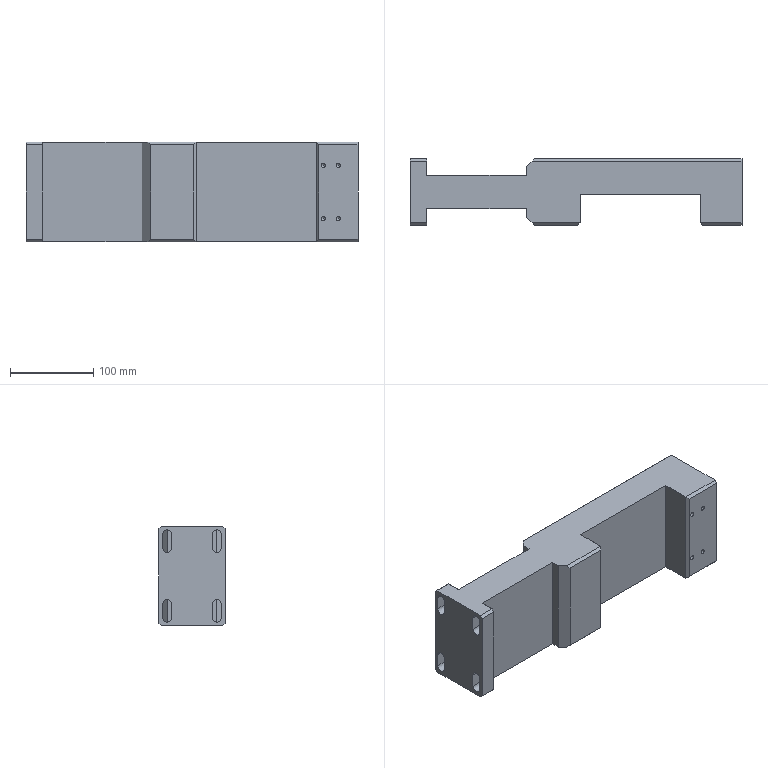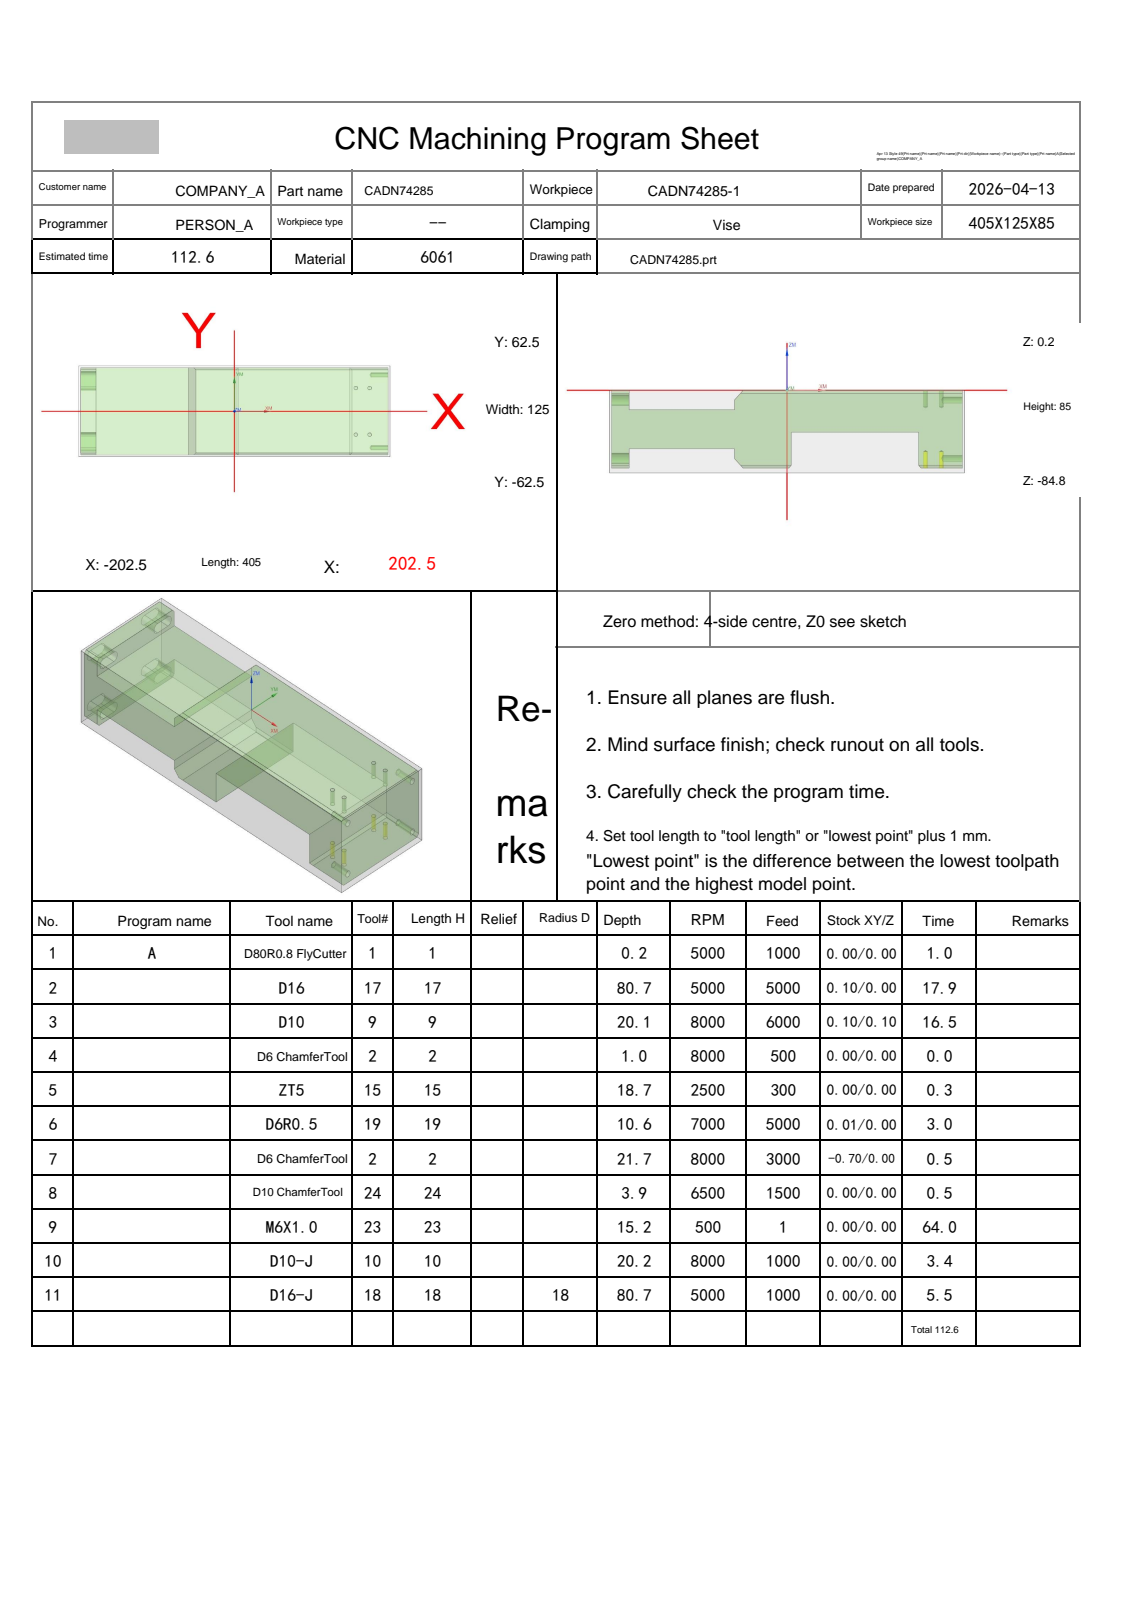NC program | NX | posted by the shop | part box 400 x 80 x 120 mm
Lines 711 to 1887 of 8047:
N3 T09 M06
(D10  D=10. R=0. H=09 ce=0.10 di=0.10)
G00 G90 G54 X-108.23 Y-74.5 M03 S8000
G43 H09 Z10.2
M08
Z.703
G01 Z-.498 F6000.
Y-67.08
G03 X-115.23 Y-60.08 I-7. J0.0
G01 X-174.823
G02 X-175.265 Y-61.98 I-5.294 J.231
X-175.856 Y-63. I-4.852 J2.13
G01 X-176.489
G02 X-180. Y-64.039 I-3.531 J5.482
G01 X-199.92
Y-63.
X-200.
Y-64.039
Y-63.
X-200.08
Y-62.639
X-200.001
X-200. Y-62.64
X-199.999 Y-62.639
X-199.92 Y-62.64
X-198.52 Y-62.639
X-180.
G03 X-174.924 Y-58.018 I-.021 J5.121
G01 X-174.843 Y-57.501
X-174.82 Y-56.969
Y-56.774
X-174.821 Y-56.579
Y-56.188
Y53.513
X-174.82 Y54.405
Y55.297
Y56.188
X-174.822 Y57.085
X-174.844 Y57.509
X-174.924 Y58.018
G03 X-180. Y62.639 I-5.096 J-.499
G01 X-198.52
X-199.92 Y62.64
X-200.08 Y62.639
Y63.
X-199.92
Y64.039
X-179.994
G02 X-176.489 Y63. I-.026 J-6.521
G01 X-175.86
G02 X-174.823 Y60.08 I-4.254 J-3.154
G01 X-174.024
X-65.178
G02 X-64.15 Y63. I5.19 J-.186
G01 X-63.921
X-64.088 Y62.761
X-64.213 Y62.557
X-64.304 Y62.395
X-64.465 Y62.064
X-64.595 Y61.736
X-64.716 Y61.351
X-64.803 Y60.967
X-64.856 Y60.637
X-64.925 Y60.09
X-64.79 Y60.08
X-58.147
G02 X-57.124 Y63. I5.489 J-.285
G01 X-54.085
G02 X-50.568 Y64.039 I3.516 J-5.432
G01 X199.92
Y63.
X200.08
Y62.639
X199.92 Y62.64
X198.52 Y62.639
X-50.568
G03 X-55.639 Y57.568 I0.0 J-5.071
G01 Y-57.568
G03 X-50.568 Y-62.639 I5.071 J0.0
G01 X199.92
X199.921
X200.08
Y-63.
X199.92
Y-64.039
X-50.568
G02 X-54.085 Y-63. I0.0 J6.471
G01 X-57.14
G02 X-57.487 Y-62.469 I4.246 J3.149
G01 X-57.719 Y-62.023
X-57.883 Y-61.559
X-58.102 Y-60.66
X-58.195 Y-60.08
X-64.79
X-64.925 Y-60.09
X-64.856 Y-60.637
X-64.822 Y-60.857
X-64.757 Y-61.187
X-64.668 Y-61.516
X-64.554 Y-61.845
X-64.414 Y-62.175
X-64.244 Y-62.504
X-64.04 Y-62.833
X-63.917 Y-63.
X-64.152
G02 X-65.178 Y-60.08 I4.162 J3.102
G01 X-112.216
G02 X-113.029 Y-59.662 I.001 J1.
G01 X-117.431 Y-53.498
G03 X-118.244 Y-53.08 I-.813 J-.582
G01 X-166.825
G02 X-167.821 Y-52.084 I.004 J1.
G01 Y52.084
G02 X-166.825 Y53.08 I1. J-.004
G01 X-65.055
X-63.635
G02 X-62.639 Y52.084 I-.004 J-1.
G01 Y-52.084
G02 X-63.635 Y-53.08 I-1. J.004
G01 X-65.178
X-112.216
G02 X-113.029 Y-52.662 I.001 J1.
G01 X-117.431 Y-46.498
G03 X-118.244 Y-46.08 I-.813 J-.582
G01 X-159.826
G02 X-160.821 Y-45.085 I.005 J1.
G01 Y45.085
G02 X-159.826 Y46.08 I1. J-.005
G01 X-70.634
G02 X-69.639 Y45.085 I-.005 J-1.
G01 Y-45.085
G02 X-70.634 Y-46.08 I-1. J.005
G01 X-112.216
G02 X-113.029 Y-45.662 I.001 J1.
G01 X-117.431 Y-39.498
G03 X-118.244 Y-39.08 I-.813 J-.582
G01 X-152.826
G02 X-153.821 Y-38.085 I.005 J1.
G01 Y38.085
G02 X-152.826 Y39.08 I1. J-.005
G01 X-77.634
G02 X-76.639 Y38.085 I-.005 J-1.
G01 Y-38.085
G02 X-77.634 Y-39.08 I-1. J.005
G01 X-112.216
G02 X-113.029 Y-38.662 I0.0 J1.
G01 X-117.431 Y-32.498
G03 X-118.244 Y-32.08 I-.813 J-.582
G01 X-145.826
G02 X-146.821 Y-31.085 I.005 J1.
G01 Y31.085
G02 X-145.826 Y32.08 I1. J-.005
G01 X-84.634
G02 X-83.639 Y31.085 I-.005 J-1.
G01 Y-31.085
G02 X-84.634 Y-32.08 I-1. J.005
G01 X-112.216
G02 X-113.029 Y-31.662 I0.0 J1.
G01 X-117.431 Y-25.498
G03 X-118.244 Y-25.08 I-.814 J-.582
G01 X-138.827
G02 X-139.821 Y-24.085 I.005 J1.
G01 Y24.085
G02 X-138.827 Y25.08 I1. J-.005
G01 X-91.634
G02 X-90.639 Y24.085 I-.005 J-1.
G01 Y-24.085
G02 X-91.634 Y-25.08 I-1. J.005
G01 X-112.216
G02 X-113.029 Y-24.662 I0.0 J1.
G01 X-117.431 Y-18.498
G03 X-118.244 Y-18.08 I-.814 J-.582
G01 X-131.827
G02 X-132.821 Y-17.085 I.005 J1.
G01 Y17.085
G02 X-131.827 Y18.08 I1. J-.005
G01 X-98.634
G02 X-97.639 Y17.085 I-.005 J-1.
G01 Y-17.085
G02 X-98.634 Y-18.08 I-1. J.005
G01 X-112.216
G02 X-113.029 Y-17.662 I0.0 J1.
G01 X-117.431 Y-11.499
G03 X-118.244 Y-11.08 I-.814 J-.581
G01 X-124.827
G02 X-125.821 Y-10.085 I.005 J1.
G01 Y10.085
G02 X-124.827 Y11.08 I1. J-.005
G01 X-105.634
G02 X-104.639 Y10.085 I-.005 J-1.
G01 Y-10.085
G02 X-105.634 Y-11.08 I-1. J.005
G01 X-112.216
G02 X-113.029 Y-10.661 I0.0 J1.
G01 X-117.47 Y-4.444
G03 X-118.052 Y-4.053 I-.814 J-.582
G02 X-118.821 Y-3.085 I.231 J.973
G01 Y3.085
G02 X-117.827 Y4.08 I1. J-.005
G01 X-112.634
G02 X-111.639 Y3.085 I-.005 J-1.
G01 Y-3.085
G02 X-112.634 Y-4.08 I-1. J.005
G01 X-115.23
X-115.73
G03 X-122.73 Y-11.08 I0.0 J-7.
G01 Z.703
G00 Z3.
G01 X-108.23 Y-74.5
G00 Z.205
G01 Z-.995
Y-67.08
G03 X-115.23 Y-60.08 I-7. J0.0
G01 X-174.823
G02 X-180.08 Y-65.148 I-5.294 J.231
G01 X-200. Y-65.151
X-200.085 Y-65.156
X-200.08 Y-65.071
Y-63.136
X-199.92
X-180.
G03 X-174.898 Y-58.014 I-.021 J5.122
G01 X-174.9 Y-57.879
X-174.843 Y-57.501
X-174.82 Y-56.969
Y-56.774
X-174.821 Y-56.579
Y-56.188
Y53.513
X-174.82 Y54.405
Y55.297
Y56.188
X-174.822 Y57.085
X-174.844 Y57.509
X-174.9 Y57.879
Y57.995
Y58.016
G03 X-180. Y63.136 I-5.121 J0.0
G01 X-199.92
X-200.
X-200.08
Y65.071
X-200.085 Y65.156
X-200. Y65.151
X-199.742
X-180.08 Y65.142
G02 X-174.823 Y60.08 I-.034 J-5.296
G01 X-65.178
G02 X-63.663 Y63.563 I5.19 J-.186
G01 X-63.563 Y63.663
X-63.503 Y63.727
X-63.447 Y63.66
X-63.385 Y63.615
X-63.438 Y63.56
X-63.529 Y63.429
X-63.71 Y63.267
X-63.836 Y63.113
X-63.964 Y62.943
X-64.088 Y62.761
X-64.213 Y62.557
X-64.304 Y62.395
X-64.465 Y62.064
X-64.595 Y61.736
X-64.716 Y61.351
X-64.803 Y60.967
X-64.856 Y60.637
X-64.925 Y60.09
X-64.79 Y60.08
X-58.147
G02 X-55.897 Y64.236 I5.489 J-.285
X-52.574 Y65.157 I3.324 J-5.531
X-52.279 Y65.151 I0.0 J-6.453
G01 X200.
X200.085 Y65.156
X200.08 Y65.071
Y63.136
X200.
X199.92
X-51.066
G03 X-56.136 Y58.066 I0.0 J-5.071
G01 Y-58.066
G03 X-51.066 Y-63.136 I5.071 J0.0
G01 X199.92
X200.08
Y-64.215
Y-65.071
X200.085 Y-65.156
X200. Y-65.151
X-52.283
X-53.179 Y-65.129
G02 X-57.487 Y-62.469 I.285 J5.279
G01 X-57.719 Y-62.023
X-57.883 Y-61.559
X-58.102 Y-60.66
X-58.195 Y-60.08
X-64.79
X-64.925 Y-60.09
X-64.856 Y-60.637
X-64.822 Y-60.857
X-64.757 Y-61.187
X-64.668 Y-61.516
X-64.554 Y-61.845
X-64.414 Y-62.175
X-64.244 Y-62.504
X-64.04 Y-62.833
X-63.799 Y-63.16
X-63.529 Y-63.428
X-63.512 Y-63.453
X-63.482 Y-63.523
X-63.443 Y-63.597
X-63.521 Y-63.627
X-63.548 Y-63.64
X-63.624 Y-63.68
X-63.655 Y-63.6
X-63.676 Y-63.553
G02 X-65.178 Y-60.08 I3.686 J3.655
G01 X-112.216
G02 X-113.029 Y-59.662 I.001 J1.
G01 X-117.431 Y-53.498
G03 X-118.244 Y-53.08 I-.813 J-.582
G01 X-166.825
G02 X-167.821 Y-52.083 I.003 J1.
G01 Y52.083
G02 X-166.825 Y53.08 I1. J-.003
G01 X-65.055
X-64.133
G02 X-63.136 Y52.083 I-.003 J-1.
G01 Y-52.083
G02 X-64.133 Y-53.08 I-1. J.003
G01 X-65.178
X-112.216
G02 X-113.029 Y-52.662 I.001 J1.
G01 X-117.431 Y-46.498
G03 X-118.244 Y-46.08 I-.813 J-.582
G01 X-159.825
G02 X-160.821 Y-45.084 I.004 J1.
G01 Y45.084
G02 X-159.825 Y46.08 I1. J-.004
G01 X-71.132
G02 X-70.136 Y45.084 I-.004 J-1.
G01 Y-45.084
G02 X-71.132 Y-46.08 I-1. J.004
G01 X-112.216
G02 X-113.029 Y-45.662 I.001 J1.
G01 X-117.431 Y-39.498
G03 X-118.244 Y-39.08 I-.813 J-.582
G01 X-152.826
G02 X-153.821 Y-38.084 I.004 J1.
G01 Y38.084
G02 X-152.826 Y39.08 I1. J-.004
G01 X-78.132
G02 X-77.136 Y38.084 I-.004 J-1.
G01 Y-38.084
G02 X-78.132 Y-39.08 I-1. J.004
G01 X-112.216
G02 X-113.029 Y-38.662 I0.0 J1.
G01 X-117.431 Y-32.498
G03 X-118.244 Y-32.08 I-.813 J-.582
G01 X-145.826
G02 X-146.821 Y-31.085 I.004 J1.
G01 Y31.084
G02 X-145.826 Y32.08 I1. J-.004
G01 X-85.132
G02 X-84.136 Y31.085 I-.004 J-1.
G01 Y-31.084
G02 X-85.132 Y-32.08 I-1. J.004
G01 X-112.216
G02 X-113.029 Y-31.662 I0.0 J1.
G01 X-117.431 Y-25.498
G03 X-118.244 Y-25.08 I-.814 J-.582
G01 X-138.826
G02 X-139.821 Y-24.085 I.005 J1.
G01 Y24.085
G02 X-138.826 Y25.08 I1. J-.005
G01 X-92.132
G02 X-91.136 Y24.085 I-.005 J-1.
G01 Y-24.085
G02 X-92.132 Y-25.08 I-1. J.005
G01 X-112.216
G02 X-113.029 Y-24.662 I0.0 J1.
G01 X-117.431 Y-18.498
G03 X-118.244 Y-18.08 I-.814 J-.582
G01 X-131.826
G02 X-132.821 Y-17.085 I.005 J1.
G01 Y17.085
G02 X-131.826 Y18.08 I1. J-.005
G01 X-99.132
G02 X-98.136 Y17.085 I-.005 J-1.
G01 Y-17.085
G02 X-99.132 Y-18.08 I-1. J.005
G01 X-112.216
G02 X-113.029 Y-17.662 I0.0 J1.
G01 X-117.431 Y-11.498
G03 X-118.244 Y-11.08 I-.814 J-.582
G01 X-124.826
G02 X-125.821 Y-10.085 I.005 J1.
G01 Y10.085
G02 X-124.826 Y11.08 I1. J-.005
G01 X-106.132
G02 X-105.136 Y10.085 I-.005 J-1.
G01 Y-10.085
G02 X-106.132 Y-11.08 I-1. J.005
G01 X-112.216
G02 X-113.029 Y-10.661 I0.0 J1.
G01 X-117.47 Y-4.444
G03 X-118.052 Y-4.053 I-.814 J-.582
G02 X-118.821 Y-3.085 I.231 J.973
G01 Y3.085
G02 X-117.826 Y4.08 I1. J-.005
G01 X-113.131
G02 X-112.136 Y3.085 I-.005 J-1.
G01 Y-3.085
G02 X-113.131 Y-4.08 I-1. J.005
G01 X-115.23
X-115.73
G03 X-122.73 Y-11.08 I0.0 J-7.
G01 Z.205
G00 Z3.
G01 X-108.23 Y-74.5
G00 Z-.293
G01 Z-1.493
Y-67.08
G03 X-115.23 Y-60.08 I-7. J0.0
G01 X-174.823
G02 X-178.055 Y-64.731 I-5.294 J.231
X-180. Y-65.034 I-1.965 J6.218
G01 X-199.92
Y-63.634
X-180.
G03 X-174.9 Y-58.513 I-.021 J5.121
G01 Y-58.492
Y-57.879
X-174.843 Y-57.501
X-174.82 Y-56.969
Y-56.774
X-174.821 Y-56.579
Y-56.188
Y53.513
X-174.82 Y54.405
Y55.297
Y56.188
X-174.822 Y57.085
X-174.844 Y57.509
X-174.9 Y57.879
Y58.492
Y58.513
G03 X-180. Y63.634 I-5.121 J0.0
G01 X-199.92
Y65.034
X-179.994
G02 X-178.105 Y64.746 I-.026 J-6.521
X-174.823 Y60.08 I-2.008 J-4.9
G01 X-65.178
G02 X-64.15 Y63. I5.19 J-.186
G01 X-63.921
X-64.088 Y62.761
X-64.213 Y62.557
X-64.304 Y62.395
X-64.465 Y62.064
X-64.595 Y61.736
X-64.716 Y61.351
X-64.803 Y60.967
X-64.856 Y60.637
X-64.925 Y60.09
X-64.79 Y60.08
X-58.147
G02 X-57.124 Y63. I5.489 J-.285
G01 X-56.273
G02 X-51.563 Y65.034 I4.71 J-4.437
G01 X199.92
Y63.634
X-51.563
G03 X-56.634 Y58.563 I0.0 J-5.071
G01 Y-58.563
G03 X-51.563 Y-63.634 I5.071 J0.0
G01 X199.92
Y-65.034
X-51.563
G02 X-56.273 Y-63. I0.0 J6.471
G01 X-57.14
G02 X-57.487 Y-62.469 I4.246 J3.149
G01 X-57.719 Y-62.023
X-57.883 Y-61.559
X-58.102 Y-60.66
X-58.195 Y-60.08
X-64.79
X-64.925 Y-60.09
X-64.856 Y-60.637
X-64.822 Y-60.857
X-64.757 Y-61.187
X-64.668 Y-61.516
X-64.554 Y-61.845
X-64.414 Y-62.175
X-64.244 Y-62.504
X-64.04 Y-62.833
X-63.917 Y-63.
X-64.152
G02 X-65.178 Y-60.08 I4.162 J3.102
G01 X-112.216
G02 X-113.029 Y-59.662 I.001 J1.
G01 X-117.431 Y-53.499
G03 X-118.244 Y-53.08 I-.813 J-.582
G01 X-166.826
G02 X-167.821 Y-52.085 I.005 J1.
G01 Y52.085
G02 X-166.826 Y53.08 I1. J-.005
G01 X-65.055
X-64.629
G02 X-63.634 Y52.085 I-.005 J-1.
G01 Y-52.085
G02 X-64.629 Y-53.08 I-1. J.005
G01 X-65.068 Y-53.081
X-112.216 Y-53.08
G02 X-113.029 Y-52.662 I.001 J1.
G01 X-117.431 Y-46.499
G03 X-118.244 Y-46.08 I-.813 J-.582
G01 X-159.827
G02 X-160.821 Y-45.085 I.005 J1.
G01 Y45.085
G02 X-159.827 Y46.08 I1. J-.005
G01 X-71.629
G02 X-70.634 Y45.085 I-.005 J-1.
G01 Y-45.086
G02 X-71.629 Y-46.081 I-1. J.005
G01 X-112.216 Y-46.08
G02 X-113.029 Y-45.662 I.001 J1.
G01 X-117.431 Y-39.499
G03 X-118.244 Y-39.08 I-.813 J-.582
G01 X-152.827
G02 X-153.821 Y-38.086 I.006 J1.
G01 Y38.086
G02 X-152.827 Y39.08 I1. J-.006
G01 X-78.628
G02 X-77.634 Y38.086 I-.006 J-1.
G01 Y-38.086
G02 X-78.628 Y-39.081 I-1. J.006
G01 X-112.216 Y-39.08
G02 X-113.029 Y-38.662 I0.0 J1.
G01 X-117.431 Y-32.499
G03 X-118.244 Y-32.08 I-.813 J-.582
G01 X-145.827
G02 X-146.821 Y-31.086 I.006 J1.
G01 Y31.086
G02 X-145.827 Y32.08 I1. J-.006
G01 X-85.628
G02 X-84.634 Y31.086 I-.006 J-1.
G01 Y-31.086
G02 X-85.628 Y-32.081 I-1. J.006
G01 X-112.216 Y-32.08
G02 X-113.029 Y-31.662 I0.0 J1.
G01 X-117.431 Y-25.499
G03 X-118.244 Y-25.08 I-.814 J-.582
G01 X-138.827
G02 X-139.821 Y-24.086 I.006 J1.
G01 Y24.086
G02 X-138.827 Y25.08 I1. J-.006
G01 X-92.628
G02 X-91.634 Y24.086 I-.006 J-1.
G01 Y-24.086
G02 X-92.628 Y-25.081 I-1. J.006
G01 X-112.216 Y-25.08
G02 X-113.029 Y-24.662 I0.0 J1.
G01 X-117.431 Y-18.499
G03 X-118.244 Y-18.08 I-.814 J-.582
G01 X-131.827
G02 X-132.821 Y-17.086 I.006 J1.
G01 Y17.086
G02 X-131.827 Y18.08 I1. J-.006
G01 X-99.628
G02 X-98.634 Y17.086 I-.006 J-1.
G01 Y-17.087
G02 X-99.628 Y-18.081 I-1. J.006
G01 X-112.216 Y-18.08
G02 X-113.029 Y-17.662 I0.0 J1.
G01 X-117.431 Y-11.499
G03 X-118.244 Y-11.08 I-.814 J-.581
G01 X-124.827
G02 X-125.821 Y-10.086 I.006 J1.
G01 Y10.086
G02 X-124.827 Y11.08 I1. J-.006
G01 X-106.628
G02 X-105.634 Y10.086 I-.006 J-1.
G01 Y-10.087
G02 X-106.628 Y-11.081 I-1. J.006
G01 X-112.215 Y-11.08
G02 X-113.029 Y-10.662 I0.0 J1.
G01 X-117.469 Y-4.445
G03 X-118.052 Y-4.054 I-.814 J-.582
G02 X-118.821 Y-3.086 I.23 J.973
G01 Y3.086
G02 X-117.827 Y4.08 I1. J-.006
G01 X-113.628
G02 X-112.634 Y3.086 I-.006 J-1.
G01 Y-3.087
G02 X-113.628 Y-4.08 I-1. J.006
G01 X-115.23
X-115.73
G03 X-122.73 Y-11.08 I0.0 J-7.
G01 Z-.293
G00 Z3.
G01 X-108.23 Y-74.5
G00 Z-.79
G01 Z-1.99
Y-67.08
G03 X-115.23 Y-60.08 I-7. J0.0
G01 X-174.823
G02 X-180.08 Y-65.148 I-5.294 J.231
G01 X-200. Y-65.151
X-200.085 Y-65.156
X-200.08 Y-65.071
Y-64.131
X-199.92
X-180.
G03 X-174.9 Y-58.99 I-.042 J5.142
G01 Y-57.879
X-174.843 Y-57.501
X-174.82 Y-56.969
Y-56.774
X-174.821 Y-56.579
Y-56.188
Y53.513
X-174.82 Y54.405
Y55.297
Y56.188
X-174.822 Y57.085
X-174.844 Y57.509
X-174.9 Y57.879
Y58.99
G03 X-180. Y64.131 I-5.142 J-.001
G01 X-199.92
X-199.997
X-200.
X-200.08
Y65.071
X-200.085 Y65.156
X-200. Y65.151
X-199.742
X-180.08 Y65.142
G02 X-174.823 Y60.08 I-.034 J-5.296
G01 X-65.178
G02 X-63.663 Y63.563 I5.19 J-.186
G01 X-63.563 Y63.663
X-63.503 Y63.727
X-63.447 Y63.66
X-63.385 Y63.615
X-63.438 Y63.56
X-63.529 Y63.429
X-63.71 Y63.267
X-63.836 Y63.113
X-63.964 Y62.943
X-64.088 Y62.761
X-64.213 Y62.557
X-64.304 Y62.395
X-64.465 Y62.064
X-64.595 Y61.736
X-64.716 Y61.351
X-64.803 Y60.967
X-64.856 Y60.637
X-64.925 Y60.09
X-64.79 Y60.08
X-58.147
G02 X-55.897 Y64.236 I5.489 J-.285
X-52.574 Y65.157 I3.324 J-5.531
X-52.279 Y65.151 I0.0 J-6.453
G01 X200.
X200.085 Y65.156
X200.08 Y65.071
Y64.131
X200.
X199.997
X199.92
X-52.061
G03 X-57.131 Y59.061 I0.0 J-5.071
G01 Y-59.061
G03 X-52.061 Y-64.131 I5.071 J0.0
G01 X199.92
X200.08
Y-65.071
X200.085 Y-65.156
X200. Y-65.151
X-52.283
X-53.179 Y-65.129
G02 X-57.487 Y-62.469 I.285 J5.279
G01 X-57.719 Y-62.023
X-57.883 Y-61.559
X-58.102 Y-60.66
X-58.195 Y-60.08
X-64.79
X-64.925 Y-60.09
X-64.856 Y-60.637
X-64.822 Y-60.857
X-64.757 Y-61.187
X-64.668 Y-61.516
X-64.554 Y-61.845
X-64.414 Y-62.175
X-64.244 Y-62.504
X-64.04 Y-62.833
X-63.799 Y-63.16
X-63.529 Y-63.428
X-63.512 Y-63.453
X-63.482 Y-63.523
X-63.443 Y-63.597
X-63.521 Y-63.627
X-63.548 Y-63.64
X-63.624 Y-63.68
X-63.655 Y-63.6
X-63.676 Y-63.553
G02 X-65.178 Y-60.08 I3.686 J3.655
G01 X-112.216
G02 X-113.029 Y-59.662 I.001 J1.
G01 X-117.431 Y-53.498
G03 X-118.244 Y-53.08 I-.813 J-.582
G01 X-166.826
G02 X-167.821 Y-52.084 I.004 J1.
G01 Y52.084
G02 X-166.826 Y53.08 I1. J-.004
G01 X-65.133
X-65.131
G02 X-64.131 Y52.085 I0.0 J-1.
G01 Y-52.085
G02 X-65.132 Y-53.081 I-1.001 J.004
G01 X-65.178 Y-53.08
X-112.216
G02 X-113.029 Y-52.662 I.001 J1.
G01 X-117.431 Y-46.498
G03 X-118.244 Y-46.08 I-.813 J-.582
G01 X-159.826
G02 X-160.821 Y-45.085 I.005 J1.
G01 Y45.085
G02 X-159.826 Y46.08 I1. J-.005
G01 X-72.126
G02 X-71.131 Y45.085 I-.005 J-1.
G01 Y-45.085
G02 X-72.126 Y-46.08 I-1. J.005
G01 X-112.216
G02 X-113.029 Y-45.662 I.001 J1.
G01 X-117.431 Y-39.498
G03 X-118.244 Y-39.08 I-.813 J-.582
G01 X-152.827
G02 X-153.821 Y-38.085 I.005 J1.
G01 Y38.085
G02 X-152.827 Y39.08 I1. J-.005
G01 X-79.126
G02 X-78.131 Y38.085 I-.005 J-1.
G01 Y-38.085
G02 X-79.126 Y-39.08 I-1. J.005
G01 X-112.216
G02 X-113.029 Y-38.662 I0.0 J1.
G01 X-117.431 Y-32.498
G03 X-118.244 Y-32.08 I-.813 J-.582
G01 X-145.827
G02 X-146.821 Y-31.085 I.005 J1.
G01 Y31.085
G02 X-145.827 Y32.08 I1. J-.005
G01 X-86.126
G02 X-85.131 Y31.085 I-.005 J-1.
G01 Y-31.085
G02 X-86.126 Y-32.08 I-1. J.005
G01 X-112.216
G02 X-113.029 Y-31.662 I0.0 J1.
G01 X-117.431 Y-25.498
G03 X-118.244 Y-25.08 I-.814 J-.582
G01 X-138.827
G02 X-139.821 Y-24.085 I.005 J1.
G01 Y24.085
G02 X-138.827 Y25.08 I1. J-.005
G01 X-93.126
G02 X-92.131 Y24.085 I-.005 J-1.
G01 Y-24.085
G02 X-93.126 Y-25.08 I-1. J.005
G01 X-112.216
G02 X-113.029 Y-24.662 I0.0 J1.
G01 X-117.431 Y-18.498
G03 X-118.244 Y-18.08 I-.814 J-.582
G01 X-131.827
G02 X-132.821 Y-17.086 I.006 J1.
G01 Y17.086
G02 X-131.827 Y18.08 I1. J-.006
G01 X-100.126
G02 X-99.131 Y17.086 I-.006 J-1.
G01 Y-17.086
G02 X-100.126 Y-18.08 I-1. J.006
G01 X-112.216
G02 X-113.029 Y-17.662 I0.0 J1.
G01 X-117.431 Y-11.499
G03 X-118.244 Y-11.08 I-.814 J-.581
G01 X-124.827
G02 X-125.821 Y-10.086 I.006 J1.
G01 Y10.086
G02 X-124.827 Y11.08 I1. J-.006
G01 X-107.126
G02 X-106.131 Y10.086 I-.006 J-1.
G01 Y-10.086
G02 X-107.126 Y-11.08 I-1. J.006
G01 X-112.216
G02 X-113.029 Y-10.661 I0.0 J1.
G01 X-117.47 Y-4.444
G03 X-118.052 Y-4.053 I-.814 J-.582
G02 X-118.821 Y-3.086 I.231 J.973
G01 Y3.086
G02 X-117.827 Y4.08 I1. J-.006
G01 X-114.126
G02 X-113.131 Y3.086 I-.006 J-1.
G01 Y-3.086
G02 X-114.126 Y-4.08 I-1. J.006
G01 X-115.23
X-115.73
G03 X-122.73 Y-11.08 I0.0 J-7.
G01 Z-.79
G00 Z3.
G01 X-108.23 Y-74.5
G00 Z-1.288
G01 Z-2.488
Y-67.08
G03 X-115.23 Y-60.08 I-7. J0.0
G01 X-174.823
G02 X-180.08 Y-65.148 I-5.294 J.231
G01 X-200. Y-65.151
X-200.085 Y-65.156
X-200.08 Y-65.071
Y-64.629
X-200.
X-199.991
X-199.92
X-180.
G03 X-174.9 Y-59.487 I-.048 J5.147
G01 Y-57.879
X-174.843 Y-57.501
X-174.82 Y-56.969
Y-56.774
X-174.821 Y-56.579
Y-56.188
Y53.513
X-174.82 Y54.405
Y55.297
Y56.188
X-174.822 Y57.085
X-174.844 Y57.509
X-174.9 Y57.879
Y59.487
G03 X-180. Y64.629 I-5.148 J-.006
G01 X-199.92
X-199.989
X-200.
X-200.08
Y65.071
X-200.085 Y65.156
X-200. Y65.151
X-199.742
X-180.08 Y65.142
G02 X-174.823 Y60.08 I-.034 J-5.296
G01 X-65.178
G02 X-63.663 Y63.563 I5.19 J-.186
G01 X-63.563 Y63.663
X-63.503 Y63.727
X-63.447 Y63.66
X-63.385 Y63.615
X-63.438 Y63.56
X-63.529 Y63.429
X-63.71 Y63.267
X-63.836 Y63.113
X-63.964 Y62.943
X-64.088 Y62.761
X-64.213 Y62.557
X-64.304 Y62.395
X-64.465 Y62.064
X-64.595 Y61.736
X-64.716 Y61.351
X-64.803 Y60.967
X-64.856 Y60.637
X-64.925 Y60.09
X-64.79 Y60.08
X-58.147
G02 X-55.897 Y64.236 I5.489 J-.285
X-52.574 Y65.157 I3.324 J-5.531
X-52.279 Y65.151 I0.0 J-6.453
G01 X200.
X200.085 Y65.156
X200.08 Y65.071
Y64.629
X200.
X199.989
X199.92
X-52.558
G03 X-57.629 Y59.558 I0.0 J-5.071
G01 Y-59.558
G03 X-52.558 Y-64.629 I5.071 J0.0
G01 X199.92
X200.08
Y-65.071
X200.085 Y-65.156
X200. Y-65.151
X-52.283
X-53.179 Y-65.129
G02 X-57.487 Y-62.469 I.285 J5.279
G01 X-57.719 Y-62.023
X-57.883 Y-61.559
X-58.102 Y-60.66
X-58.195 Y-60.08
X-64.79
X-64.925 Y-60.09
X-64.856 Y-60.637
X-64.822 Y-60.857
X-64.757 Y-61.187
X-64.668 Y-61.516
X-64.554 Y-61.845
X-64.414 Y-62.175
X-64.244 Y-62.504
X-64.04 Y-62.833
X-63.799 Y-63.16
X-63.529 Y-63.428
X-63.512 Y-63.453
X-63.482 Y-63.523
X-63.443 Y-63.597
X-63.521 Y-63.627
X-63.548 Y-63.64
X-63.624 Y-63.68
X-63.655 Y-63.6
X-63.676 Y-63.553
G02 X-65.178 Y-60.08 I3.686 J3.655
G01 X-112.216
G02 X-113.029 Y-59.662 I.001 J1.
G01 X-117.431 Y-53.498
G03 X-118.244 Y-53.08 I-.813 J-.582
G01 X-166.826
G02 X-167.821 Y-52.085 I.005 J1.
G01 Y52.085
G02 X-166.826 Y53.08 I1. J-.005
G01 X-65.624
G02 X-64.629 Y52.085 I-.005 J-1.
G01 Y-52.085
G02 X-65.624 Y-53.08 I-1. J.005
G01 X-112.216
G02 X-113.029 Y-52.662 I.001 J1.
G01 X-117.431 Y-46.498
G03 X-118.244 Y-46.08 I-.813 J-.582
G01 X-159.827
G02 X-160.821 Y-45.085 I.005 J1.
G01 Y45.085
G02 X-159.827 Y46.08 I1. J-.005
G01 X-72.624
G02 X-71.629 Y45.085 I-.005 J-1.
G01 Y-45.085
G02 X-72.624 Y-46.08 I-1. J.005
G01 X-112.216
G02 X-113.029 Y-45.662 I.001 J1.
G01 X-117.431 Y-39.498
G03 X-118.244 Y-39.08 I-.813 J-.582
G01 X-152.827
G02 X-153.821 Y-38.085 I.005 J1.
G01 Y38.085
G02 X-152.827 Y39.08 I1. J-.005
G01 X-79.623
G02 X-78.629 Y38.086 I-.005 J-1.
G01 Y-38.086
G02 X-79.623 Y-39.08 I-1. J.005
G01 X-112.216
G02 X-113.029 Y-38.662 I0.0 J1.
G01 X-117.431 Y-32.498
G03 X-118.244 Y-32.08 I-.813 J-.582
G01 X-145.827
G02 X-146.821 Y-31.086 I.006 J1.
G01 Y31.086
G02 X-145.827 Y32.08 I1. J-.006
G01 X-86.623
G02 X-85.629 Y31.086 I-.006 J-1.
G01 Y-31.086
G02 X-86.623 Y-32.08 I-1. J.006
G01 X-112.216
G02 X-113.029 Y-31.662 I0.0 J1.
G01 X-117.431 Y-25.498
G03 X-118.244 Y-25.08 I-.814 J-.582
G01 X-138.827
G02 X-139.821 Y-24.086 I.006 J1.
G01 Y24.086
G02 X-138.827 Y25.08 I1. J-.006
G01 X-93.623
G02 X-92.629 Y24.086 I-.006 J-1.
G01 Y-24.086
G02 X-93.623 Y-25.08 I-1. J.006
G01 X-112.216
G02 X-113.029 Y-24.662 I0.0 J1.
G01 X-117.431 Y-18.498
G03 X-118.244 Y-18.08 I-.814 J-.582
G01 X-131.827
G02 X-132.821 Y-17.086 I.006 J1.
G01 Y17.086
G02 X-131.827 Y18.08 I1. J-.006
G01 X-100.623
G02 X-99.629 Y17.086 I-.006 J-1.
G01 Y-17.086
G02 X-100.623 Y-18.08 I-1. J.006
G01 X-112.216
G02 X-113.029 Y-17.662 I0.0 J1.
G01 X-117.431 Y-11.499
G03 X-118.244 Y-11.08 I-.814 J-.581
G01 X-124.827
G02 X-125.821 Y-10.086 I.006 J1.
G01 Y10.086
G02 X-124.827 Y11.08 I1. J-.006
G01 X-107.623
G02 X-106.629 Y10.086 I-.006 J-1.
G01 Y-10.086
G02 X-107.623 Y-11.08 I-1. J.006
G01 X-112.216
G02 X-113.029 Y-10.661 I0.0 J1.
G01 X-117.47 Y-4.444
G03 X-118.052 Y-4.053 I-.814 J-.582
G02 X-118.821 Y-3.086 I.231 J.973
G01 Y3.086
G02 X-117.827 Y4.08 I1. J-.006
G01 X-114.623
G02 X-113.629 Y3.086 I-.006 J-1.
G01 Y-3.086
G02 X-114.623 Y-4.08 I-1. J.006
G01 X-115.23
X-115.73
G03 X-122.73 Y-11.08 I0.0 J-7.
G01 Z-1.288
G00 Z3.
G01 X-108.23 Y-74.5
G00 Z-1.785
G01 Z-2.985
Y-67.08
G03 X-115.23 Y-60.08 I-7. J0.0
G01 X-174.823
G02 X-175.856 Y-63. I-5.294 J.231
X-176.838 Y-64.012 I-4.26 J3.151
G01 X-176.898 Y-63.939
X-176.479 Y-63.591
X-176.394 Y-63.506
G03 X-174.9 Y-59.9 I-3.606 J3.606
G01 Y-57.879
X-174.843 Y-57.501
X-174.833 Y-57.298
X-174.82 Y-56.969
Y-56.774
X-174.821 Y-56.579
Y-56.188
Y53.513
X-174.82 Y54.405
Y55.297
Y56.188
X-174.822 Y57.085
X-174.832 Y57.293
X-174.844 Y57.509
X-174.9 Y57.879
Y59.9
G03 X-176.394 Y63.506 I-5.1 J0.0
G01 X-176.479 Y63.591
X-176.93 Y63.966
G03 X-177.242 Y64.201 I-3.178 J-3.887
G01 X-177.197 Y64.266
G02 X-175.86 Y63. I-2.917 J-4.42
X-174.823 Y60.08 I-4.254 J-3.154
G01 X-65.178
G02 X-64.15 Y63. I5.19 J-.186
G01 X-63.921
X-64.088 Y62.761
X-64.213 Y62.557
X-64.304 Y62.395
X-64.465 Y62.064
X-64.595 Y61.736
X-64.716 Y61.351
X-64.803 Y60.967
X-64.856 Y60.637
X-64.925 Y60.09
X-64.79 Y60.08
X-58.147
X-58.127 Y59.921
Y59.92
X-58.126 Y-60.037
X-58.195 Y-60.08
X-64.79
X-64.925 Y-60.09
X-64.856 Y-60.637
X-64.822 Y-60.857
X-64.757 Y-61.187
X-64.668 Y-61.516
X-64.554 Y-61.845
X-64.414 Y-62.175
X-64.244 Y-62.504
X-64.04 Y-62.833
X-63.917 Y-63.
X-64.152
G02 X-65.178 Y-60.08 I4.162 J3.102
G01 X-112.216
G02 X-113.029 Y-59.662 I0.0 J1.
G01 X-117.431 Y-53.498
G03 X-118.244 Y-53.08 I-.813 J-.582
G01 X-166.827
G02 X-167.821 Y-52.086 I.006 J1.
G01 Y52.086
G02 X-166.827 Y53.08 I1. J-.006
G01 X-66.121
G02 X-65.126 Y52.086 I-.006 J-1.
G01 Y-52.086
G02 X-66.121 Y-53.08 I-1. J.006
G01 X-112.216
G02 X-113.029 Y-52.662 I.001 J1.
G01 X-117.431 Y-46.498
G03 X-118.244 Y-46.08 I-.813 J-.582
G01 X-159.827
G02 X-160.821 Y-45.086 I.006 J1.
G01 Y45.086
G02 X-159.827 Y46.08 I1. J-.006
G01 X-73.121
G02 X-72.126 Y45.086 I-.006 J-1.
G01 Y-45.086
G02 X-73.121 Y-46.08 I-1. J.006
G01 X-112.216
G02 X-113.029 Y-45.662 I0.0 J1.
G01 X-117.431 Y-39.498
G03 X-118.244 Y-39.08 I-.813 J-.582
G01 X-152.827
G02 X-153.821 Y-38.086 I.006 J1.
G01 Y38.086
G02 X-152.827 Y39.08 I1. J-.006
G01 X-80.12
G02 X-79.126 Y38.086 I-.006 J-1.
G01 Y-38.086
G02 X-80.12 Y-39.08 I-1. J.006
G01 X-112.216
G02 X-113.029 Y-38.662 I0.0 J1.
G01 X-117.431 Y-32.498
G03 X-118.244 Y-32.08 I-.813 J-.582
G01 X-145.828
G02 X-146.821 Y-31.086 I.006 J1.
G01 Y31.086
G02 X-145.828 Y32.08 I1. J-.006
G01 X-87.12
G02 X-86.126 Y31.086 I-.006 J-1.
G01 Y-31.086
G02 X-87.12 Y-32.08 I-1. J.006
G01 X-112.216
G02 X-113.029 Y-31.662 I0.0 J1.
G01 X-117.431 Y-25.498
G03 X-118.244 Y-25.08 I-.813 J-.582
G01 X-138.828
G02 X-139.821 Y-24.086 I.006 J1.
G01 Y24.086
G02 X-138.828 Y25.08 I1. J-.006
G01 X-94.12
G02 X-93.126 Y24.086 I-.006 J-1.
G01 Y-24.086
G02 X-94.12 Y-25.08 I-1. J.006
G01 X-112.216
G02 X-113.029 Y-24.662 I0.0 J1.
G01 X-117.431 Y-18.498
G03 X-118.244 Y-18.08 I-.814 J-.582
G01 X-131.828
G02 X-132.821 Y-17.086 I.006 J1.
G01 Y17.086
G02 X-131.828 Y18.08 I1. J-.006
G01 X-101.12
G02 X-100.126 Y17.086 I-.006 J-1.
G01 Y-17.086
G02 X-101.12 Y-18.08 I-1. J.006
G01 X-112.216
G02 X-113.029 Y-17.662 I0.0 J1.
G01 X-117.431 Y-11.499
G03 X-118.244 Y-11.08 I-.814 J-.581
G01 X-124.828
G02 X-125.821 Y-10.086 I.006 J1.
G01 Y10.086
G02 X-124.828 Y11.08 I1. J-.006
G01 X-108.12
G02 X-107.126 Y10.086 I-.006 J-1.
G01 Y-10.086
G02 X-108.12 Y-11.08 I-1. J.006
G01 X-112.216
G02 X-113.029 Y-10.661 I0.0 J1.
G01 X-117.47 Y-4.444
G03 X-118.052 Y-4.053 I-.814 J-.582
G02 X-118.821 Y-3.087 I.231 J.973
G01 Y3.087
G02 X-117.828 Y4.08 I1. J-.006